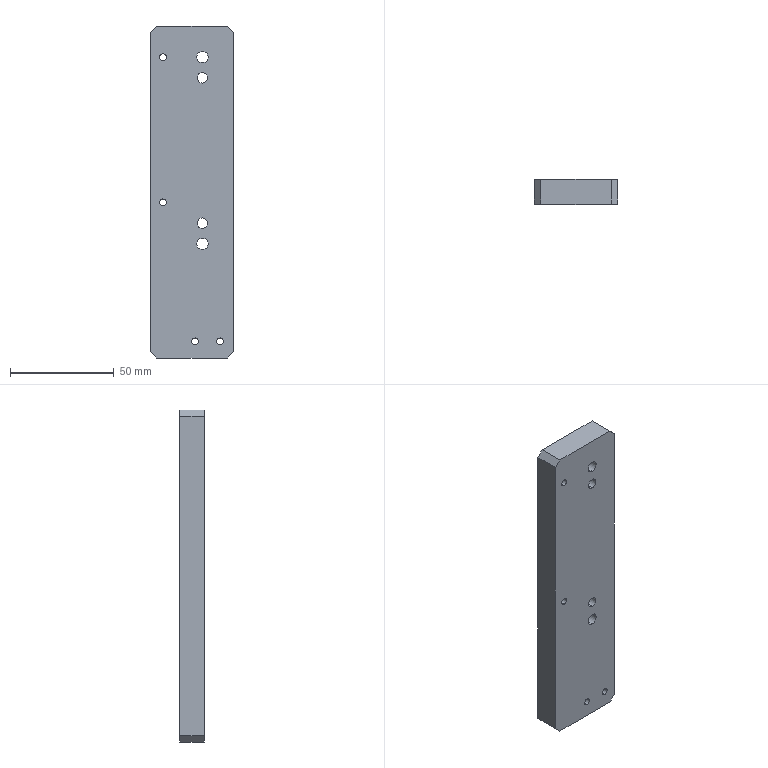Part | STEP file | PN_0051 | 1 solid | 40 faces | box 40 x 12 x 160 mm | volume 74451 mm3 | cylinder 24 | plane 12 | cone 4 | commonest cylinder face diameters 3.3 x8 3 x4 5 x4 5.5 x4 10 x4